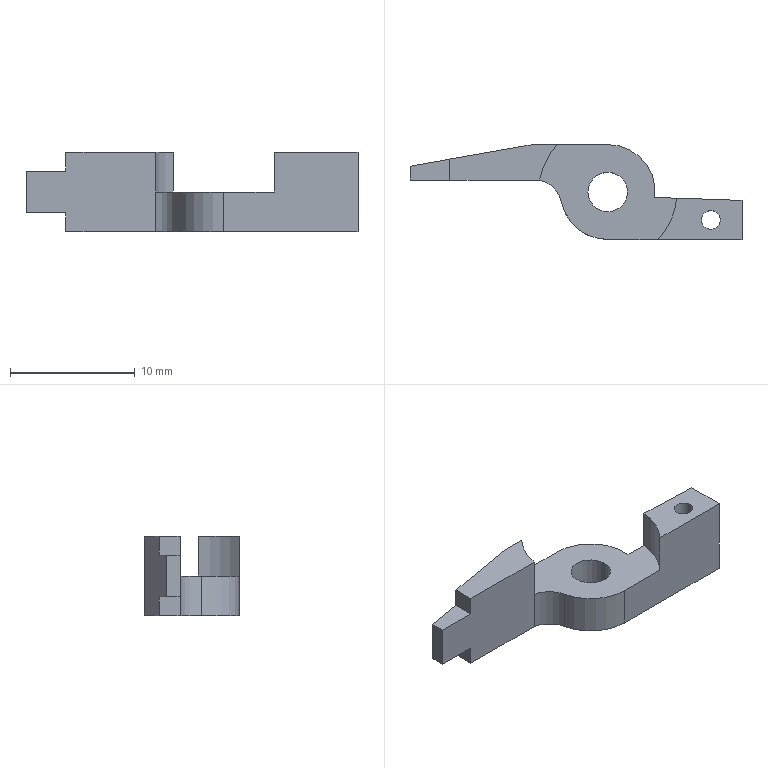Part | SolidWorks | features ICE 6, Scale 2, Extrusion 1 | 1 solid | 24 faces | box 26.652 x 7.62 x 6.35 mm | volume 402.278 mm3 | plane 15 | cylinder 9 | commonest cylinder face diameters 1.5 x2 3.175 x2 7.62 x2 11.115 x2 4.445 x1
STEP:
#1=CARTESIAN_POINT('',(7.527,-2.245,0.));
#2=VERTEX_POINT('',#1);
#3=CARTESIAN_POINT('',(9.027,-2.245,0.));
#4=VERTEX_POINT('',#3);
#5=CARTESIAN_POINT('',(8.277,-2.245,0.));
#6=DIRECTION('',(0.,0.,1.));
#7=DIRECTION('',(1.,0.,0.));
#8=AXIS2_PLACEMENT_3D('',#5,#6,#7);
#9=CIRCLE('',#8,0.75);
#10=EDGE_CURVE('',#2,#4,#9,.T.);
#11=ORIENTED_EDGE('',*,*,#10,.F.);
#12=CARTESIAN_POINT('',(7.527,-2.245,6.35));
#13=VERTEX_POINT('',#12);
#14=CARTESIAN_POINT('',(7.527,-2.245,0.));
#15=DIRECTION('',(0.,0.,1.));
#16=VECTOR('',#15,1000.);
#17=LINE('',#14,#16);
#18=EDGE_CURVE('',#2,#13,#17,.T.);
#19=ORIENTED_EDGE('',*,*,#18,.T.);
#20=CARTESIAN_POINT('',(9.027,-2.245,6.35));
#21=VERTEX_POINT('',#20);
#22=CARTESIAN_POINT('',(8.277,-2.245,6.35));
#23=DIRECTION('',(0.,0.,1.));
#24=DIRECTION('',(1.,0.,0.));
#25=AXIS2_PLACEMENT_3D('',#22,#23,#24);
#26=CIRCLE('',#25,0.75);
#27=EDGE_CURVE('',#13,#21,#26,.T.);
#28=ORIENTED_EDGE('',*,*,#27,.T.);
#29=CARTESIAN_POINT('',(9.027,-2.245,0.));
#30=DIRECTION('',(0.,0.,1.));
#31=VECTOR('',#30,1000.);
#32=LINE('',#29,#31);
#33=EDGE_CURVE('',#4,#21,#32,.T.);
#34=ORIENTED_EDGE('',*,*,#33,.F.);
#35=EDGE_LOOP('',(#11,#19,#28,#34));
#36=FACE_OUTER_BOUND('',#35,.T.);
#37=CARTESIAN_POINT('',(8.277,-2.245,0.));
#38=DIRECTION('',(0.,0.,1.));
#39=DIRECTION('',(1.,0.,0.));
#40=AXIS2_PLACEMENT_3D('',#37,#38,#39);
#41=CYLINDRICAL_SURFACE('',#40,0.75);
#42=ADVANCED_FACE('',(#36),#41,.F.);
#43=CARTESIAN_POINT('',(-1.587,0.,3.175));
#44=VERTEX_POINT('',#43);
#45=CARTESIAN_POINT('',(1.587,0.,3.175));
#46=VERTEX_POINT('',#45);
#47=CARTESIAN_POINT('',(0.,0.,3.175));
#48=DIRECTION('',(0.,0.,1.));
#49=DIRECTION('',(1.,0.,0.));
#50=AXIS2_PLACEMENT_3D('',#47,#48,#49);
#51=CIRCLE('',#50,1.587);
#52=EDGE_CURVE('',#44,#46,#51,.T.);
#53=ORIENTED_EDGE('',*,*,#52,.T.);
#54=CARTESIAN_POINT('',(1.587,0.,0.));
#55=VERTEX_POINT('',#54);
#56=CARTESIAN_POINT('',(1.587,0.,6.35));
#57=DIRECTION('',(0.,0.,-1.));
#58=VECTOR('',#57,1000.);
#59=LINE('',#56,#58);
#60=EDGE_CURVE('',#46,#55,#59,.T.);
#61=ORIENTED_EDGE('',*,*,#60,.T.);
#62=CARTESIAN_POINT('',(-1.587,0.,0.));
#63=VERTEX_POINT('',#62);
#64=CARTESIAN_POINT('',(0.,0.,0.));
#65=DIRECTION('',(0.,0.,1.));
#66=DIRECTION('',(1.,0.,0.));
#67=AXIS2_PLACEMENT_3D('',#64,#65,#66);
#68=CIRCLE('',#67,1.587);
#69=EDGE_CURVE('',#63,#55,#68,.T.);
#70=ORIENTED_EDGE('',*,*,#69,.F.);
#71=CARTESIAN_POINT('',(-1.587,0.,6.35));
#72=DIRECTION('',(0.,0.,-1.));
#73=VECTOR('',#72,1000.);
#74=LINE('',#71,#73);
#75=EDGE_CURVE('',#44,#63,#74,.T.);
#76=ORIENTED_EDGE('',*,*,#75,.F.);
#77=EDGE_LOOP('',(#53,#61,#70,#76));
#78=FACE_OUTER_BOUND('',#77,.T.);
#79=CARTESIAN_POINT('',(0.,0.,6.35));
#80=DIRECTION('',(0.,0.,-1.));
#81=DIRECTION('',(-1.,0.,0.));
#82=AXIS2_PLACEMENT_3D('',#79,#80,#81);
#83=CYLINDRICAL_SURFACE('',#82,1.587);
#84=ADVANCED_FACE('',(#78),#83,.F.);
#85=CARTESIAN_POINT('',(-15.875,2.065,4.85));
#86=VERTEX_POINT('',#85);
#87=CARTESIAN_POINT('',(-15.875,2.065,1.5));
#88=VERTEX_POINT('',#87);
#89=CARTESIAN_POINT('',(-15.875,2.065,6.35));
#90=DIRECTION('',(0.,0.,-1.));
#91=VECTOR('',#90,1000.);
#92=LINE('',#89,#91);
#93=EDGE_CURVE('',#86,#88,#92,.T.);
#94=ORIENTED_EDGE('',*,*,#93,.T.);
#95=CARTESIAN_POINT('',(-15.875,0.9525,1.5));
#96=VERTEX_POINT('',#95);
#97=CARTESIAN_POINT('',(-15.875,2.065,1.5));
#98=DIRECTION('',(0.,1.,0.));
#99=VECTOR('',#98,1000.);
#100=LINE('',#97,#99);
#101=EDGE_CURVE('',#96,#88,#100,.T.);
#102=ORIENTED_EDGE('',*,*,#101,.F.);
#103=CARTESIAN_POINT('',(-15.875,0.9525,4.85));
#104=VERTEX_POINT('',#103);
#105=CARTESIAN_POINT('',(-15.875,0.9525,-3.315));
#106=DIRECTION('',(0.,0.,1.));
#107=VECTOR('',#106,1000.);
#108=LINE('',#105,#107);
#109=EDGE_CURVE('',#96,#104,#108,.T.);
#110=ORIENTED_EDGE('',*,*,#109,.T.);
#111=CARTESIAN_POINT('',(-15.875,2.065,4.85));
#112=DIRECTION('',(0.,-1.,0.));
#113=VECTOR('',#112,1000.);
#114=LINE('',#111,#113);
#115=EDGE_CURVE('',#86,#104,#114,.T.);
#116=ORIENTED_EDGE('',*,*,#115,.F.);
#117=EDGE_LOOP('',(#94,#102,#110,#116));
#118=FACE_OUTER_BOUND('',#117,.T.);
#119=CARTESIAN_POINT('',(-15.875,0.,6.35));
#120=DIRECTION('',(1.,0.,0.));
#121=DIRECTION('',(0.,0.,-1.));
#122=AXIS2_PLACEMENT_3D('',#119,#120,#121);
#123=PLANE('',#122);
#124=ADVANCED_FACE('',(#118),#123,.F.);
#125=CARTESIAN_POINT('',(-5.475,0.9525,3.175));
#126=VERTEX_POINT('',#125);
#127=CARTESIAN_POINT('',(-3.73,-0.7755,3.175));
#128=VERTEX_POINT('',#127);
#129=CARTESIAN_POINT('',(-5.906,-1.228,3.175));
#130=DIRECTION('',(0.,0.,-1.));
#131=DIRECTION('',(1.,0.,0.));
#132=AXIS2_PLACEMENT_3D('',#129,#130,#131);
#133=CIRCLE('',#132,2.223);
#134=EDGE_CURVE('',#126,#128,#133,.T.);
#135=ORIENTED_EDGE('',*,*,#134,.F.);
#136=CARTESIAN_POINT('',(-5.475,0.9525,0.));
#137=VERTEX_POINT('',#136);
#138=CARTESIAN_POINT('',(-5.475,0.9525,6.35));
#139=DIRECTION('',(0.,0.,-1.));
#140=VECTOR('',#139,1000.);
#141=LINE('',#138,#140);
#142=EDGE_CURVE('',#126,#137,#141,.T.);
#143=ORIENTED_EDGE('',*,*,#142,.T.);
#144=CARTESIAN_POINT('',(-3.73,-0.7755,0.));
#145=VERTEX_POINT('',#144);
#146=CARTESIAN_POINT('',(-5.906,-1.228,0.));
#147=DIRECTION('',(0.,0.,-1.));
#148=DIRECTION('',(1.,0.,0.));
#149=AXIS2_PLACEMENT_3D('',#146,#147,#148);
#150=CIRCLE('',#149,2.223);
#151=EDGE_CURVE('',#137,#145,#150,.T.);
#152=ORIENTED_EDGE('',*,*,#151,.T.);
#153=CARTESIAN_POINT('',(-3.73,-0.7755,6.35));
#154=DIRECTION('',(0.,0.,-1.));
#155=VECTOR('',#154,1000.);
#156=LINE('',#153,#155);
#157=EDGE_CURVE('',#128,#145,#156,.T.);
#158=ORIENTED_EDGE('',*,*,#157,.F.);
#159=EDGE_LOOP('',(#135,#143,#152,#158));
#160=FACE_OUTER_BOUND('',#159,.T.);
#161=CARTESIAN_POINT('',(-5.906,-1.228,6.35));
#162=DIRECTION('',(0.,0.,-1.));
#163=DIRECTION('',(-1.,0.,0.));
#164=AXIS2_PLACEMENT_3D('',#161,#162,#163);
#165=CYLINDRICAL_SURFACE('',#164,2.223);
#166=ADVANCED_FACE('',(#160),#165,.F.);
#167=CARTESIAN_POINT('',(0.,-3.81,3.175));
#168=VERTEX_POINT('',#167);
#169=CARTESIAN_POINT('',(0.,0.,3.175));
#170=DIRECTION('',(0.,0.,1.));
#171=DIRECTION('',(1.,0.,0.));
#172=AXIS2_PLACEMENT_3D('',#169,#170,#171);
#173=CIRCLE('',#172,3.81);
#174=EDGE_CURVE('',#128,#168,#173,.T.);
#175=ORIENTED_EDGE('',*,*,#174,.F.);
#176=ORIENTED_EDGE('',*,*,#157,.T.);
#177=CARTESIAN_POINT('',(0.,-3.81,0.));
#178=VERTEX_POINT('',#177);
#179=CARTESIAN_POINT('',(0.,0.,0.));
#180=DIRECTION('',(0.,0.,1.));
#181=DIRECTION('',(1.,0.,0.));
#182=AXIS2_PLACEMENT_3D('',#179,#180,#181);
#183=CIRCLE('',#182,3.81);
#184=EDGE_CURVE('',#145,#178,#183,.T.);
#185=ORIENTED_EDGE('',*,*,#184,.T.);
#186=CARTESIAN_POINT('',(0.,-3.81,6.35));
#187=DIRECTION('',(0.,0.,-1.));
#188=VECTOR('',#187,1000.);
#189=LINE('',#186,#188);
#190=EDGE_CURVE('',#168,#178,#189,.T.);
#191=ORIENTED_EDGE('',*,*,#190,.F.);
#192=EDGE_LOOP('',(#175,#176,#185,#191));
#193=FACE_OUTER_BOUND('',#192,.T.);
#194=CARTESIAN_POINT('',(0.,0.,6.35));
#195=DIRECTION('',(0.,0.,-1.));
#196=DIRECTION('',(-1.,0.,0.));
#197=AXIS2_PLACEMENT_3D('',#194,#195,#196);
#198=CYLINDRICAL_SURFACE('',#197,3.81);
#199=ADVANCED_FACE('',(#193),#198,.T.);
#200=CARTESIAN_POINT('',(3.785,-0.4358,3.175));
#201=VERTEX_POINT('',#200);
#202=CARTESIAN_POINT('',(0.,3.81,3.175));
#203=VERTEX_POINT('',#202);
#204=CARTESIAN_POINT('',(0.,0.,3.175));
#205=DIRECTION('',(0.,0.,1.));
#206=DIRECTION('',(1.,0.,0.));
#207=AXIS2_PLACEMENT_3D('',#204,#205,#206);
#208=CIRCLE('',#207,3.81);
#209=EDGE_CURVE('',#201,#203,#208,.T.);
#210=ORIENTED_EDGE('',*,*,#209,.F.);
#211=CARTESIAN_POINT('',(3.785,-0.4358,0.));
#212=VERTEX_POINT('',#211);
#213=CARTESIAN_POINT('',(3.785,-0.4358,6.35));
#214=DIRECTION('',(0.,0.,-1.));
#215=VECTOR('',#214,1000.);
#216=LINE('',#213,#215);
#217=EDGE_CURVE('',#201,#212,#216,.T.);
#218=ORIENTED_EDGE('',*,*,#217,.T.);
#219=CARTESIAN_POINT('',(0.,3.81,0.));
#220=VERTEX_POINT('',#219);
#221=CARTESIAN_POINT('',(0.,0.,0.));
#222=DIRECTION('',(0.,0.,1.));
#223=DIRECTION('',(1.,0.,0.));
#224=AXIS2_PLACEMENT_3D('',#221,#222,#223);
#225=CIRCLE('',#224,3.81);
#226=EDGE_CURVE('',#212,#220,#225,.T.);
#227=ORIENTED_EDGE('',*,*,#226,.T.);
#228=CARTESIAN_POINT('',(0.,3.81,6.35));
#229=DIRECTION('',(0.,0.,-1.));
#230=VECTOR('',#229,1000.);
#231=LINE('',#228,#230);
#232=EDGE_CURVE('',#203,#220,#231,.T.);
#233=ORIENTED_EDGE('',*,*,#232,.F.);
#234=EDGE_LOOP('',(#210,#218,#227,#233));
#235=FACE_OUTER_BOUND('',#234,.T.);
#236=CARTESIAN_POINT('',(0.,0.,6.35));
#237=DIRECTION('',(0.,0.,-1.));
#238=DIRECTION('',(-1.,0.,0.));
#239=AXIS2_PLACEMENT_3D('',#236,#237,#238);
#240=CYLINDRICAL_SURFACE('',#239,3.81);
#241=ADVANCED_FACE('',(#235),#240,.T.);
#242=ORIENTED_EDGE('',*,*,#60,.F.);
#243=CARTESIAN_POINT('',(0.,0.,3.175));
#244=DIRECTION('',(0.,0.,1.));
#245=DIRECTION('',(1.,0.,0.));
#246=AXIS2_PLACEMENT_3D('',#243,#244,#245);
#247=CIRCLE('',#246,1.587);
#248=EDGE_CURVE('',#46,#44,#247,.T.);
#249=ORIENTED_EDGE('',*,*,#248,.T.);
#250=ORIENTED_EDGE('',*,*,#75,.T.);
#251=CARTESIAN_POINT('',(0.,0.,0.));
#252=DIRECTION('',(0.,0.,1.));
#253=DIRECTION('',(1.,0.,0.));
#254=AXIS2_PLACEMENT_3D('',#251,#252,#253);
#255=CIRCLE('',#254,1.587);
#256=EDGE_CURVE('',#55,#63,#255,.T.);
#257=ORIENTED_EDGE('',*,*,#256,.F.);
#258=EDGE_LOOP('',(#242,#249,#250,#257));
#259=FACE_OUTER_BOUND('',#258,.T.);
#260=CARTESIAN_POINT('',(0.,0.,6.35));
#261=DIRECTION('',(0.,0.,-1.));
#262=DIRECTION('',(-1.,0.,0.));
#263=AXIS2_PLACEMENT_3D('',#260,#261,#262);
#264=CYLINDRICAL_SURFACE('',#263,1.587);
#265=ADVANCED_FACE('',(#259),#264,.F.);
#266=CARTESIAN_POINT('',(-12.675,0.9525,6.35));
#267=VERTEX_POINT('',#266);
#268=CARTESIAN_POINT('',(-12.675,2.63,6.35));
#269=VERTEX_POINT('',#268);
#270=CARTESIAN_POINT('',(-12.675,0.9525,6.35));
#271=DIRECTION('',(0.,1.,0.));
#272=VECTOR('',#271,1000.);
#273=LINE('',#270,#272);
#274=EDGE_CURVE('',#267,#269,#273,.T.);
#275=ORIENTED_EDGE('',*,*,#274,.F.);
#276=CARTESIAN_POINT('',(-5.475,0.9525,6.35));
#277=VERTEX_POINT('',#276);
#278=CARTESIAN_POINT('',(0.,0.9525,6.35));
#279=DIRECTION('',(1.,0.,0.));
#280=VECTOR('',#279,1000.);
#281=LINE('',#278,#280);
#282=EDGE_CURVE('',#267,#277,#281,.T.);
#283=ORIENTED_EDGE('',*,*,#282,.T.);
#284=CARTESIAN_POINT('',(-4.046,3.81,6.35));
#285=VERTEX_POINT('',#284);
#286=CARTESIAN_POINT('',(0.,0.,6.35));
#287=DIRECTION('',(0.,0.,1.));
#288=DIRECTION('',(1.,0.,0.));
#289=AXIS2_PLACEMENT_3D('',#286,#287,#288);
#290=CIRCLE('',#289,5.558);
#291=EDGE_CURVE('',#285,#277,#290,.T.);
#292=ORIENTED_EDGE('',*,*,#291,.F.);
#293=CARTESIAN_POINT('',(-6.,3.81,6.35));
#294=VERTEX_POINT('',#293);
#295=CARTESIAN_POINT('',(0.,3.81,6.35));
#296=DIRECTION('',(-1.,0.,0.));
#297=VECTOR('',#296,1000.);
#298=LINE('',#295,#297);
#299=EDGE_CURVE('',#285,#294,#298,.T.);
#300=ORIENTED_EDGE('',*,*,#299,.T.);
#301=CARTESIAN_POINT('',(-0.8346,4.723,6.35));
#302=DIRECTION('',(-0.9847,-0.174,0.));
#303=VECTOR('',#302,1000.);
#304=LINE('',#301,#303);
#305=EDGE_CURVE('',#294,#269,#304,.T.);
#306=ORIENTED_EDGE('',*,*,#305,.T.);
#307=EDGE_LOOP('',(#275,#283,#292,#300,#306));
#308=FACE_OUTER_BOUND('',#307,.T.);
#309=CARTESIAN_POINT('',(0.,0.,6.35));
#310=DIRECTION('',(0.,0.,1.));
#311=DIRECTION('',(1.,0.,0.));
#312=AXIS2_PLACEMENT_3D('',#309,#310,#311);
#313=PLANE('',#312);
#314=ADVANCED_FACE('',(#308),#313,.T.);
#315=CARTESIAN_POINT('',(-12.675,0.9525,1.5));
#316=VERTEX_POINT('',#315);
#317=CARTESIAN_POINT('',(-12.675,0.9525,1.5));
#318=DIRECTION('',(-1.,0.,0.));
#319=VECTOR('',#318,1000.);
#320=LINE('',#317,#319);
#321=EDGE_CURVE('',#316,#96,#320,.T.);
#322=ORIENTED_EDGE('',*,*,#321,.F.);
#323=CARTESIAN_POINT('',(-12.675,0.9525,0.));
#324=VERTEX_POINT('',#323);
#325=CARTESIAN_POINT('',(-12.675,0.9525,1.5));
#326=DIRECTION('',(0.,0.,-1.));
#327=VECTOR('',#326,1000.);
#328=LINE('',#325,#327);
#329=EDGE_CURVE('',#316,#324,#328,.T.);
#330=ORIENTED_EDGE('',*,*,#329,.T.);
#331=CARTESIAN_POINT('',(0.,0.9525,0.));
#332=DIRECTION('',(1.,0.,0.));
#333=VECTOR('',#332,1000.);
#334=LINE('',#331,#333);
#335=EDGE_CURVE('',#324,#137,#334,.T.);
#336=ORIENTED_EDGE('',*,*,#335,.T.);
#337=ORIENTED_EDGE('',*,*,#142,.F.);
#338=CARTESIAN_POINT('',(-5.475,0.9525,6.35));
#339=DIRECTION('',(0.,0.,-1.));
#340=VECTOR('',#339,1000.);
#341=LINE('',#338,#340);
#342=EDGE_CURVE('',#277,#126,#341,.T.);
#343=ORIENTED_EDGE('',*,*,#342,.F.);
#344=ORIENTED_EDGE('',*,*,#282,.F.);
#345=CARTESIAN_POINT('',(-12.675,0.9525,4.85));
#346=VERTEX_POINT('',#345);
#347=CARTESIAN_POINT('',(-12.675,0.9525,4.85));
#348=DIRECTION('',(0.,0.,1.));
#349=VECTOR('',#348,1000.);
#350=LINE('',#347,#349);
#351=EDGE_CURVE('',#346,#267,#350,.T.);
#352=ORIENTED_EDGE('',*,*,#351,.F.);
#353=CARTESIAN_POINT('',(-15.875,0.9525,4.85));
#354=DIRECTION('',(1.,0.,0.));
#355=VECTOR('',#354,1000.);
#356=LINE('',#353,#355);
#357=EDGE_CURVE('',#104,#346,#356,.T.);
#358=ORIENTED_EDGE('',*,*,#357,.F.);
#359=ORIENTED_EDGE('',*,*,#109,.F.);
#360=EDGE_LOOP('',(#322,#330,#336,#337,#343,#344,#352,#358,#359));
#361=FACE_OUTER_BOUND('',#360,.T.);
#362=CARTESIAN_POINT('',(0.,0.9525,6.35));
#363=DIRECTION('',(0.,1.,0.));
#364=DIRECTION('',(0.,0.,1.));
#365=AXIS2_PLACEMENT_3D('',#362,#363,#364);
#366=PLANE('',#365);
#367=ADVANCED_FACE('',(#361),#366,.F.);
#368=CARTESIAN_POINT('',(10.777,-3.81,0.));
#369=VERTEX_POINT('',#368);
#370=CARTESIAN_POINT('',(10.777,-3.81,6.35));
#371=VERTEX_POINT('',#370);
#372=CARTESIAN_POINT('',(10.777,-3.81,-0.00025));
#373=DIRECTION('',(0.,0.,1.));
#374=VECTOR('',#373,1000.);
#375=LINE('',#372,#374);
#376=EDGE_CURVE('',#369,#371,#375,.T.);
#377=ORIENTED_EDGE('',*,*,#376,.T.);
#378=CARTESIAN_POINT('',(4.046,-3.81,6.35));
#379=VERTEX_POINT('',#378);
#380=CARTESIAN_POINT('',(0.,-3.81,6.35));
#381=DIRECTION('',(-1.,0.,0.));
#382=VECTOR('',#381,1000.);
#383=LINE('',#380,#382);
#384=EDGE_CURVE('',#371,#379,#383,.T.);
#385=ORIENTED_EDGE('',*,*,#384,.T.);
#386=CARTESIAN_POINT('',(4.046,-3.81,3.175));
#387=VERTEX_POINT('',#386);
#388=CARTESIAN_POINT('',(4.046,-3.81,3.175));
#389=DIRECTION('',(0.,0.,1.));
#390=VECTOR('',#389,1000.);
#391=LINE('',#388,#390);
#392=EDGE_CURVE('',#387,#379,#391,.T.);
#393=ORIENTED_EDGE('',*,*,#392,.F.);
#394=CARTESIAN_POINT('',(0.,-3.81,3.175));
#395=DIRECTION('',(-1.,0.,0.));
#396=VECTOR('',#395,1000.);
#397=LINE('',#394,#396);
#398=EDGE_CURVE('',#387,#168,#397,.T.);
#399=ORIENTED_EDGE('',*,*,#398,.T.);
#400=ORIENTED_EDGE('',*,*,#190,.T.);
#401=CARTESIAN_POINT('',(0.,-3.81,0.));
#402=DIRECTION('',(-1.,0.,0.));
#403=VECTOR('',#402,1000.);
#404=LINE('',#401,#403);
#405=EDGE_CURVE('',#369,#178,#404,.T.);
#406=ORIENTED_EDGE('',*,*,#405,.F.);
#407=EDGE_LOOP('',(#377,#385,#393,#399,#400,#406));
#408=FACE_OUTER_BOUND('',#407,.T.);
#409=CARTESIAN_POINT('',(0.,-3.81,6.35));
#410=DIRECTION('',(0.,-1.,0.));
#411=DIRECTION('',(1.,0.,0.));
#412=AXIS2_PLACEMENT_3D('',#409,#410,#411);
#413=PLANE('',#412);
#414=ADVANCED_FACE('',(#408),#413,.T.);
#415=CARTESIAN_POINT('',(10.777,-0.68,6.35));
#416=VERTEX_POINT('',#415);
#417=CARTESIAN_POINT('',(5.535,-0.4969,6.35));
#418=VERTEX_POINT('',#417);
#419=CARTESIAN_POINT('',(-0.01059,-0.3033,6.35));
#420=DIRECTION('',(-0.9994,0.0349,0.));
#421=VECTOR('',#420,1000.);
#422=LINE('',#419,#421);
#423=EDGE_CURVE('',#416,#418,#422,.T.);
#424=ORIENTED_EDGE('',*,*,#423,.F.);
#425=CARTESIAN_POINT('',(10.777,-0.68,0.));
#426=VERTEX_POINT('',#425);
#427=CARTESIAN_POINT('',(10.777,-0.68,-0.00025));
#428=DIRECTION('',(0.,0.,1.));
#429=VECTOR('',#428,1000.);
#430=LINE('',#427,#429);
#431=EDGE_CURVE('',#426,#416,#430,.T.);
#432=ORIENTED_EDGE('',*,*,#431,.F.);
#433=CARTESIAN_POINT('',(-0.01059,-0.3033,0.));
#434=DIRECTION('',(-0.9994,0.0349,0.));
#435=VECTOR('',#434,1000.);
#436=LINE('',#433,#435);
#437=EDGE_CURVE('',#426,#212,#436,.T.);
#438=ORIENTED_EDGE('',*,*,#437,.T.);
#439=ORIENTED_EDGE('',*,*,#217,.F.);
#440=CARTESIAN_POINT('',(5.535,-0.4969,3.175));
#441=VERTEX_POINT('',#440);
#442=CARTESIAN_POINT('',(-0.01059,-0.3033,3.175));
#443=DIRECTION('',(-0.9994,0.0349,0.));
#444=VECTOR('',#443,1000.);
#445=LINE('',#442,#444);
#446=EDGE_CURVE('',#441,#201,#445,.T.);
#447=ORIENTED_EDGE('',*,*,#446,.F.);
#448=CARTESIAN_POINT('',(5.535,-0.4969,3.175));
#449=DIRECTION('',(0.,0.,1.));
#450=VECTOR('',#449,1000.);
#451=LINE('',#448,#450);
#452=EDGE_CURVE('',#441,#418,#451,.T.);
#453=ORIENTED_EDGE('',*,*,#452,.T.);
#454=EDGE_LOOP('',(#424,#432,#438,#439,#447,#453));
#455=FACE_OUTER_BOUND('',#454,.T.);
#456=CARTESIAN_POINT('',(-0.01059,-0.3033,6.35));
#457=DIRECTION('',(-0.0349,-0.9994,0.));
#458=DIRECTION('',(0.9994,-0.0349,0.));
#459=AXIS2_PLACEMENT_3D('',#456,#457,#458);
#460=PLANE('',#459);
#461=ADVANCED_FACE('',(#455),#460,.F.);
#462=ORIENTED_EDGE('',*,*,#299,.F.);
#463=CARTESIAN_POINT('',(-4.046,3.81,3.175));
#464=VERTEX_POINT('',#463);
#465=CARTESIAN_POINT('',(-4.046,3.81,3.175));
#466=DIRECTION('',(0.,0.,-1.));
#467=VECTOR('',#466,1000.);
#468=LINE('',#465,#467);
#469=EDGE_CURVE('',#285,#464,#468,.T.);
#470=ORIENTED_EDGE('',*,*,#469,.T.);
#471=CARTESIAN_POINT('',(0.,3.81,3.175));
#472=DIRECTION('',(-1.,0.,0.));
#473=VECTOR('',#472,1000.);
#474=LINE('',#471,#473);
#475=EDGE_CURVE('',#203,#464,#474,.T.);
#476=ORIENTED_EDGE('',*,*,#475,.F.);
#477=ORIENTED_EDGE('',*,*,#232,.T.);
#478=CARTESIAN_POINT('',(-6.,3.81,0.));
#479=VERTEX_POINT('',#478);
#480=CARTESIAN_POINT('',(0.,3.81,0.));
#481=DIRECTION('',(-1.,0.,0.));
#482=VECTOR('',#481,1000.);
#483=LINE('',#480,#482);
#484=EDGE_CURVE('',#220,#479,#483,.T.);
#485=ORIENTED_EDGE('',*,*,#484,.T.);
#486=CARTESIAN_POINT('',(-6.,3.81,6.35));
#487=DIRECTION('',(0.,0.,-1.));
#488=VECTOR('',#487,1000.);
#489=LINE('',#486,#488);
#490=EDGE_CURVE('',#294,#479,#489,.T.);
#491=ORIENTED_EDGE('',*,*,#490,.F.);
#492=EDGE_LOOP('',(#462,#470,#476,#477,#485,#491));
#493=FACE_OUTER_BOUND('',#492,.T.);
#494=CARTESIAN_POINT('',(0.,3.81,6.35));
#495=DIRECTION('',(0.,-1.,0.));
#496=DIRECTION('',(1.,0.,0.));
#497=AXIS2_PLACEMENT_3D('',#494,#495,#496);
#498=PLANE('',#497);
#499=ADVANCED_FACE('',(#493),#498,.F.);
#500=CARTESIAN_POINT('',(-12.675,2.63,0.));
#501=VERTEX_POINT('',#500);
#502=CARTESIAN_POINT('',(-0.8346,4.723,0.));
#503=DIRECTION('',(-0.9847,-0.174,0.));
#504=VECTOR('',#503,1000.);
#505=LINE('',#502,#504);
#506=EDGE_CURVE('',#479,#501,#505,.T.);
#507=ORIENTED_EDGE('',*,*,#506,.T.);
#508=CARTESIAN_POINT('',(-12.675,2.63,1.5));
#509=VERTEX_POINT('',#508);
#510=CARTESIAN_POINT('',(-12.675,2.63,1.5));
#511=DIRECTION('',(0.,0.,-1.));
#512=VECTOR('',#511,1000.);
#513=LINE('',#510,#512);
#514=EDGE_CURVE('',#509,#501,#513,.T.);
#515=ORIENTED_EDGE('',*,*,#514,.F.);
#516=CARTESIAN_POINT('',(-12.675,2.63,1.5));
#517=DIRECTION('',(0.9847,0.174,0.));
#518=VECTOR('',#517,1000.);
#519=LINE('',#516,#518);
#520=EDGE_CURVE('',#88,#509,#519,.T.);
#521=ORIENTED_EDGE('',*,*,#520,.F.);
#522=ORIENTED_EDGE('',*,*,#93,.F.);
#523=CARTESIAN_POINT('',(-12.675,2.63,4.85));
#524=VERTEX_POINT('',#523);
#525=CARTESIAN_POINT('',(-12.675,2.63,4.85));
#526=DIRECTION('',(-0.9847,-0.174,0.));
#527=VECTOR('',#526,1000.);
#528=LINE('',#525,#527);
#529=EDGE_CURVE('',#524,#86,#528,.T.);
#530=ORIENTED_EDGE('',*,*,#529,.F.);
#531=CARTESIAN_POINT('',(-12.675,2.63,4.85));
#532=DIRECTION('',(0.,0.,1.));
#533=VECTOR('',#532,1000.);
#534=LINE('',#531,#533);
#535=EDGE_CURVE('',#524,#269,#534,.T.);
#536=ORIENTED_EDGE('',*,*,#535,.T.);
#537=ORIENTED_EDGE('',*,*,#305,.F.);
#538=ORIENTED_EDGE('',*,*,#490,.T.);
#539=EDGE_LOOP('',(#507,#515,#521,#522,#530,#536,#537,#538));
#540=FACE_OUTER_BOUND('',#539,.T.);
#541=CARTESIAN_POINT('',(-0.8346,4.723,6.35));
#542=DIRECTION('',(0.174,-0.9847,0.));
#543=DIRECTION('',(0.9847,0.174,0.));
#544=AXIS2_PLACEMENT_3D('',#541,#542,#543);
#545=PLANE('',#544);
#546=ADVANCED_FACE('',(#540),#545,.F.);
#547=CARTESIAN_POINT('',(8.277,-2.245,6.35));
#548=DIRECTION('',(0.,0.,1.));
#549=DIRECTION('',(1.,0.,0.));
#550=AXIS2_PLACEMENT_3D('',#547,#548,#549);
#551=CIRCLE('',#550,0.75);
#552=EDGE_CURVE('',#21,#13,#551,.T.);
#553=ORIENTED_EDGE('',*,*,#552,.F.);
#554=ORIENTED_EDGE('',*,*,#27,.F.);
#555=EDGE_LOOP('',(#553,#554));
#556=FACE_BOUND('',#555,.T.);
#557=CARTESIAN_POINT('',(10.777,-3.81,6.35));
#558=DIRECTION('',(0.,-1.,0.));
#559=VECTOR('',#558,1000.);
#560=LINE('',#557,#559);
#561=EDGE_CURVE('',#416,#371,#560,.T.);
#562=ORIENTED_EDGE('',*,*,#561,.F.);
#563=ORIENTED_EDGE('',*,*,#423,.T.);
#564=CARTESIAN_POINT('',(0.,0.,6.35));
#565=DIRECTION('',(0.,0.,1.));
#566=DIRECTION('',(1.,0.,0.));
#567=AXIS2_PLACEMENT_3D('',#564,#565,#566);
#568=CIRCLE('',#567,5.558);
#569=EDGE_CURVE('',#379,#418,#568,.T.);
#570=ORIENTED_EDGE('',*,*,#569,.F.);
#571=ORIENTED_EDGE('',*,*,#384,.F.);
#572=EDGE_LOOP('',(#562,#563,#570,#571));
#573=FACE_OUTER_BOUND('',#572,.T.);
#574=CARTESIAN_POINT('',(0.,0.,6.35));
#575=DIRECTION('',(0.,0.,1.));
#576=DIRECTION('',(1.,0.,0.));
#577=AXIS2_PLACEMENT_3D('',#574,#575,#576);
#578=PLANE('',#577);
#579=ADVANCED_FACE('',(#556,#573),#578,.T.);
#580=CARTESIAN_POINT('',(8.277,-2.245,0.));
#581=DIRECTION('',(0.,0.,1.));
#582=DIRECTION('',(1.,0.,0.));
#583=AXIS2_PLACEMENT_3D('',#580,#581,#582);
#584=CIRCLE('',#583,0.75);
#585=EDGE_CURVE('',#4,#2,#584,.T.);
#586=ORIENTED_EDGE('',*,*,#585,.T.);
#587=ORIENTED_EDGE('',*,*,#10,.T.);
#588=EDGE_LOOP('',(#586,#587));
#589=FACE_BOUND('',#588,.T.);
#590=ORIENTED_EDGE('',*,*,#69,.T.);
#591=ORIENTED_EDGE('',*,*,#256,.T.);
#592=EDGE_LOOP('',(#590,#591));
#593=FACE_BOUND('',#592,.T.);
#594=ORIENTED_EDGE('',*,*,#335,.F.);
#595=CARTESIAN_POINT('',(-12.675,2.63,0.));
#596=DIRECTION('',(0.,-1.,0.));
#597=VECTOR('',#596,1000.);
#598=LINE('',#595,#597);
#599=EDGE_CURVE('',#501,#324,#598,.T.);
#600=ORIENTED_EDGE('',*,*,#599,.F.);
#601=ORIENTED_EDGE('',*,*,#506,.F.);
#602=ORIENTED_EDGE('',*,*,#484,.F.);
#603=ORIENTED_EDGE('',*,*,#226,.F.);
#604=ORIENTED_EDGE('',*,*,#437,.F.);
#605=CARTESIAN_POINT('',(10.777,-3.81,0.));
#606=DIRECTION('',(0.,1.,0.));
#607=VECTOR('',#606,1000.);
#608=LINE('',#605,#607);
#609=EDGE_CURVE('',#369,#426,#608,.T.);
#610=ORIENTED_EDGE('',*,*,#609,.F.);
#611=ORIENTED_EDGE('',*,*,#405,.T.);
#612=ORIENTED_EDGE('',*,*,#184,.F.);
#613=ORIENTED_EDGE('',*,*,#151,.F.);
#614=EDGE_LOOP('',(#594,#600,#601,#602,#603,#604,#610,#611,#612,#613));
#615=FACE_OUTER_BOUND('',#614,.T.);
#616=CARTESIAN_POINT('',(0.,0.,0.));
#617=DIRECTION('',(0.,0.,1.));
#618=DIRECTION('',(1.,0.,0.));
#619=AXIS2_PLACEMENT_3D('',#616,#617,#618);
#620=PLANE('',#619);
#621=ADVANCED_FACE('',(#589,#593,#615),#620,.F.);
#622=ORIENTED_EDGE('',*,*,#52,.F.);
#623=ORIENTED_EDGE('',*,*,#248,.F.);
#624=EDGE_LOOP('',(#622,#623));
#625=FACE_BOUND('',#624,.T.);
#626=ORIENTED_EDGE('',*,*,#134,.T.);
#627=ORIENTED_EDGE('',*,*,#174,.T.);
#628=ORIENTED_EDGE('',*,*,#398,.F.);
#629=CARTESIAN_POINT('',(0.,0.,3.175));
#630=DIRECTION('',(0.,0.,1.));
#631=DIRECTION('',(1.,0.,0.));
#632=AXIS2_PLACEMENT_3D('',#629,#630,#631);
#633=CIRCLE('',#632,5.558);
#634=EDGE_CURVE('',#387,#441,#633,.T.);
#635=ORIENTED_EDGE('',*,*,#634,.T.);
#636=ORIENTED_EDGE('',*,*,#446,.T.);
#637=ORIENTED_EDGE('',*,*,#209,.T.);
#638=ORIENTED_EDGE('',*,*,#475,.T.);
#639=CARTESIAN_POINT('',(0.,0.,3.175));
#640=DIRECTION('',(0.,0.,1.));
#641=DIRECTION('',(1.,0.,0.));
#642=AXIS2_PLACEMENT_3D('',#639,#640,#641);
#643=CIRCLE('',#642,5.558);
#644=EDGE_CURVE('',#464,#126,#643,.T.);
#645=ORIENTED_EDGE('',*,*,#644,.T.);
#646=EDGE_LOOP('',(#626,#627,#628,#635,#636,#637,#638,#645));
#647=FACE_OUTER_BOUND('',#646,.T.);
#648=CARTESIAN_POINT('',(0.,0.,3.175));
#649=DIRECTION('',(0.,0.,1.));
#650=DIRECTION('',(1.,0.,0.));
#651=AXIS2_PLACEMENT_3D('',#648,#649,#650);
#652=PLANE('',#651);
#653=ADVANCED_FACE('',(#625,#647),#652,.T.);
#654=ORIENTED_EDGE('',*,*,#644,.F.);
#655=ORIENTED_EDGE('',*,*,#469,.F.);
#656=ORIENTED_EDGE('',*,*,#291,.T.);
#657=ORIENTED_EDGE('',*,*,#342,.T.);
#658=EDGE_LOOP('',(#654,#655,#656,#657));
#659=FACE_OUTER_BOUND('',#658,.T.);
#660=CARTESIAN_POINT('',(0.,0.,3.175));
#661=DIRECTION('',(0.,0.,1.));
#662=DIRECTION('',(1.,0.,0.));
#663=AXIS2_PLACEMENT_3D('',#660,#661,#662);
#664=CYLINDRICAL_SURFACE('',#663,5.558);
#665=ADVANCED_FACE('',(#659),#664,.F.);
#666=ORIENTED_EDGE('',*,*,#392,.T.);
#667=ORIENTED_EDGE('',*,*,#569,.T.);
#668=ORIENTED_EDGE('',*,*,#452,.F.);
#669=ORIENTED_EDGE('',*,*,#634,.F.);
#670=EDGE_LOOP('',(#666,#667,#668,#669));
#671=FACE_OUTER_BOUND('',#670,.T.);
#672=CARTESIAN_POINT('',(0.,0.,3.175));
#673=DIRECTION('',(0.,0.,1.));
#674=DIRECTION('',(1.,0.,0.));
#675=AXIS2_PLACEMENT_3D('',#672,#673,#674);
#676=CYLINDRICAL_SURFACE('',#675,5.558);
#677=ADVANCED_FACE('',(#671),#676,.F.);
#678=ORIENTED_EDGE('',*,*,#609,.T.);
#679=ORIENTED_EDGE('',*,*,#431,.T.);
#680=ORIENTED_EDGE('',*,*,#561,.T.);
#681=ORIENTED_EDGE('',*,*,#376,.F.);
#682=EDGE_LOOP('',(#678,#679,#680,#681));
#683=FACE_OUTER_BOUND('',#682,.T.);
#684=CARTESIAN_POINT('',(10.777,-3.81,-0.00025));
#685=DIRECTION('',(-1.,0.,0.));
#686=DIRECTION('',(0.,-1.,0.));
#687=AXIS2_PLACEMENT_3D('',#684,#685,#686);
#688=PLANE('',#687);
#689=ADVANCED_FACE('',(#683),#688,.F.);
#690=ORIENTED_EDGE('',*,*,#18,.F.);
#691=ORIENTED_EDGE('',*,*,#585,.F.);
#692=ORIENTED_EDGE('',*,*,#33,.T.);
#693=ORIENTED_EDGE('',*,*,#552,.T.);
#694=EDGE_LOOP('',(#690,#691,#692,#693));
#695=FACE_OUTER_BOUND('',#694,.T.);
#696=CARTESIAN_POINT('',(8.277,-2.245,0.));
#697=DIRECTION('',(0.,0.,1.));
#698=DIRECTION('',(1.,0.,0.));
#699=AXIS2_PLACEMENT_3D('',#696,#697,#698);
#700=CYLINDRICAL_SURFACE('',#699,0.75);
#701=ADVANCED_FACE('',(#695),#700,.F.);
#702=ORIENTED_EDGE('',*,*,#274,.T.);
#703=ORIENTED_EDGE('',*,*,#535,.F.);
#704=CARTESIAN_POINT('',(-12.675,0.9525,4.85));
#705=DIRECTION('',(0.,1.,0.));
#706=VECTOR('',#705,1000.);
#707=LINE('',#704,#706);
#708=EDGE_CURVE('',#346,#524,#707,.T.);
#709=ORIENTED_EDGE('',*,*,#708,.F.);
#710=ORIENTED_EDGE('',*,*,#351,.T.);
#711=EDGE_LOOP('',(#702,#703,#709,#710));
#712=FACE_OUTER_BOUND('',#711,.T.);
#713=CARTESIAN_POINT('',(-12.675,0.9525,4.85));
#714=DIRECTION('',(1.,0.,0.));
#715=DIRECTION('',(0.,0.,-1.));
#716=AXIS2_PLACEMENT_3D('',#713,#714,#715);
#717=PLANE('',#716);
#718=ADVANCED_FACE('',(#712),#717,.F.);
#719=ORIENTED_EDGE('',*,*,#529,.T.);
#720=ORIENTED_EDGE('',*,*,#115,.T.);
#721=ORIENTED_EDGE('',*,*,#357,.T.);
#722=ORIENTED_EDGE('',*,*,#708,.T.);
#723=EDGE_LOOP('',(#719,#720,#721,#722));
#724=FACE_OUTER_BOUND('',#723,.T.);
#725=CARTESIAN_POINT('',(0.,0.,4.85));
#726=DIRECTION('',(0.,0.,1.));
#727=DIRECTION('',(1.,0.,0.));
#728=AXIS2_PLACEMENT_3D('',#725,#726,#727);
#729=PLANE('',#728);
#730=ADVANCED_FACE('',(#724),#729,.T.);
#731=ORIENTED_EDGE('',*,*,#599,.T.);
#732=ORIENTED_EDGE('',*,*,#329,.F.);
#733=CARTESIAN_POINT('',(-12.675,2.63,1.5));
#734=DIRECTION('',(0.,-1.,0.));
#735=VECTOR('',#734,1000.);
#736=LINE('',#733,#735);
#737=EDGE_CURVE('',#509,#316,#736,.T.);
#738=ORIENTED_EDGE('',*,*,#737,.F.);
#739=ORIENTED_EDGE('',*,*,#514,.T.);
#740=EDGE_LOOP('',(#731,#732,#738,#739));
#741=FACE_OUTER_BOUND('',#740,.T.);
#742=CARTESIAN_POINT('',(-12.675,2.63,1.5));
#743=DIRECTION('',(1.,0.,0.));
#744=DIRECTION('',(0.,0.,-1.));
#745=AXIS2_PLACEMENT_3D('',#742,#743,#744);
#746=PLANE('',#745);
#747=ADVANCED_FACE('',(#741),#746,.F.);
#748=ORIENTED_EDGE('',*,*,#520,.T.);
#749=ORIENTED_EDGE('',*,*,#737,.T.);
#750=ORIENTED_EDGE('',*,*,#321,.T.);
#751=ORIENTED_EDGE('',*,*,#101,.T.);
#752=EDGE_LOOP('',(#748,#749,#750,#751));
#753=FACE_OUTER_BOUND('',#752,.T.);
#754=CARTESIAN_POINT('',(0.,0.,1.5));
#755=DIRECTION('',(0.,0.,1.));
#756=DIRECTION('',(1.,0.,0.));
#757=AXIS2_PLACEMENT_3D('',#754,#755,#756);
#758=PLANE('',#757);
#759=ADVANCED_FACE('',(#753),#758,.F.);
#760=CLOSED_SHELL('',(#42,#84,#124,#166,#199,#241,#265,#314,#367,#414,#461,#499,#546,#579,#621,#653,#665,#677,#689,#701,#718,#730,#747,#759));
#761=MANIFOLD_SOLID_BREP('',#760);
#762=CARTESIAN_POINT('',(0.,0.,0.));
#763=DIRECTION('',(0.,0.,1.));
#764=DIRECTION('',(1.,0.,0.));
#765=AXIS2_PLACEMENT_3D('',#762,#763,#764);
#766=(LENGTH_UNIT()NAMED_UNIT(*)SI_UNIT(.MILLI.,.METRE.));
#767=UNCERTAINTY_MEASURE_WITH_UNIT(LENGTH_MEASURE(0.00001),#766,'','');
#768=(NAMED_UNIT(*)PLANE_ANGLE_UNIT()SI_UNIT($,.RADIAN.));
#769=(NAMED_UNIT(*)SI_UNIT($,.STERADIAN.)SOLID_ANGLE_UNIT());
#770=(GEOMETRIC_REPRESENTATION_CONTEXT(3)GLOBAL_UNCERTAINTY_ASSIGNED_CONTEXT((#767))GLOBAL_UNIT_ASSIGNED_CONTEXT((#766,#768,#769))REPRESENTATION_CONTEXT('',''));
#771=ADVANCED_BREP_SHAPE_REPRESENTATION('',(#761,#765),#770);